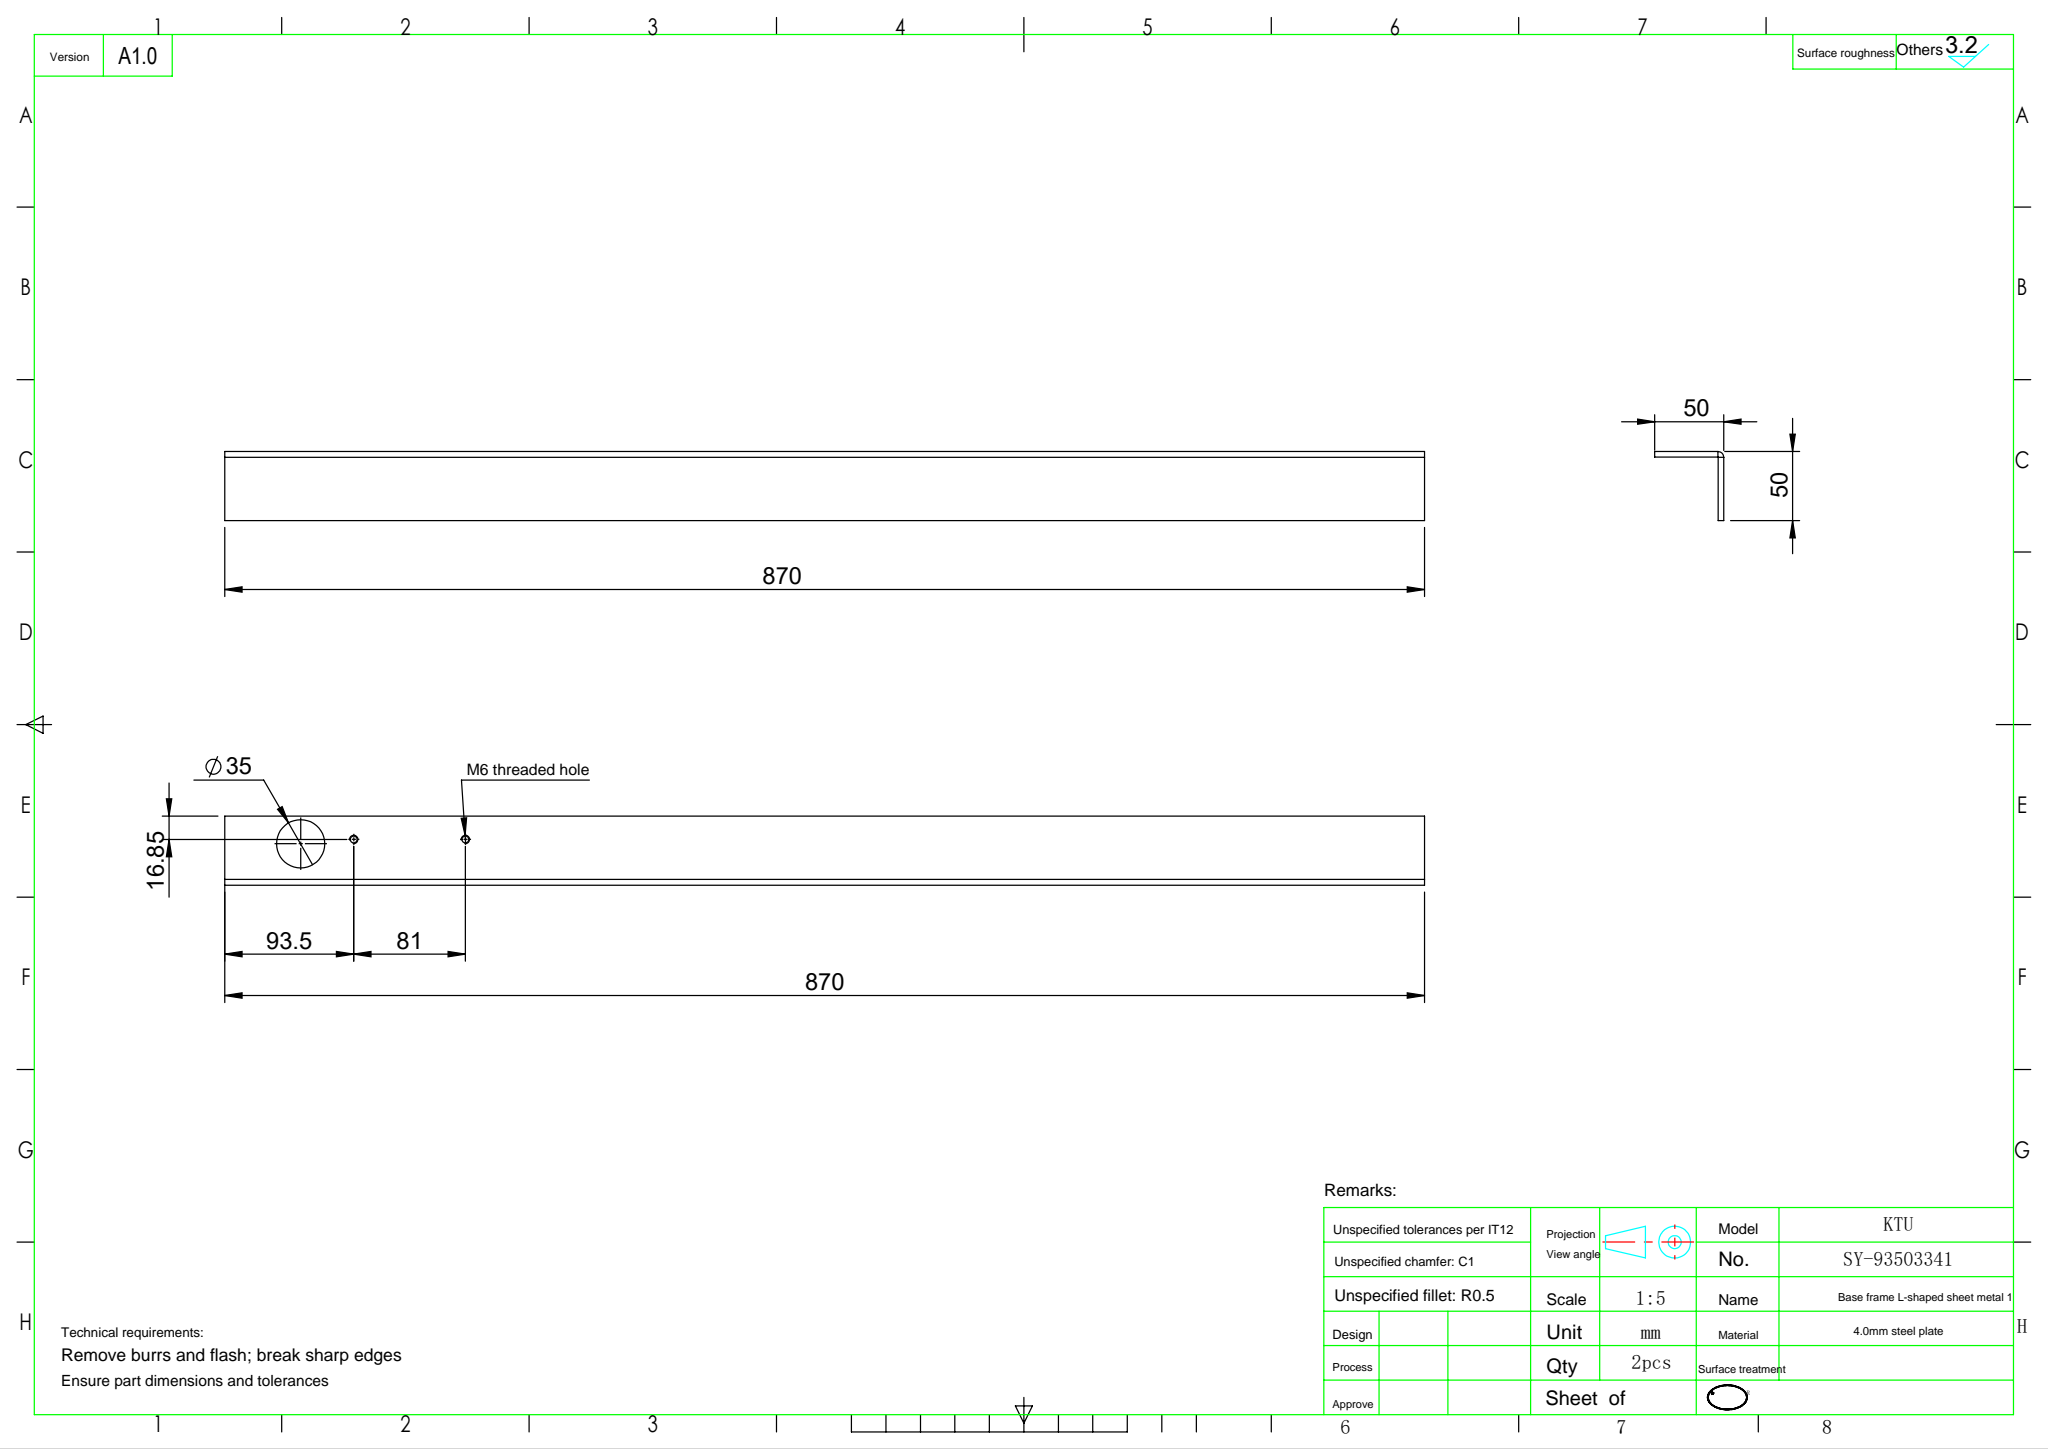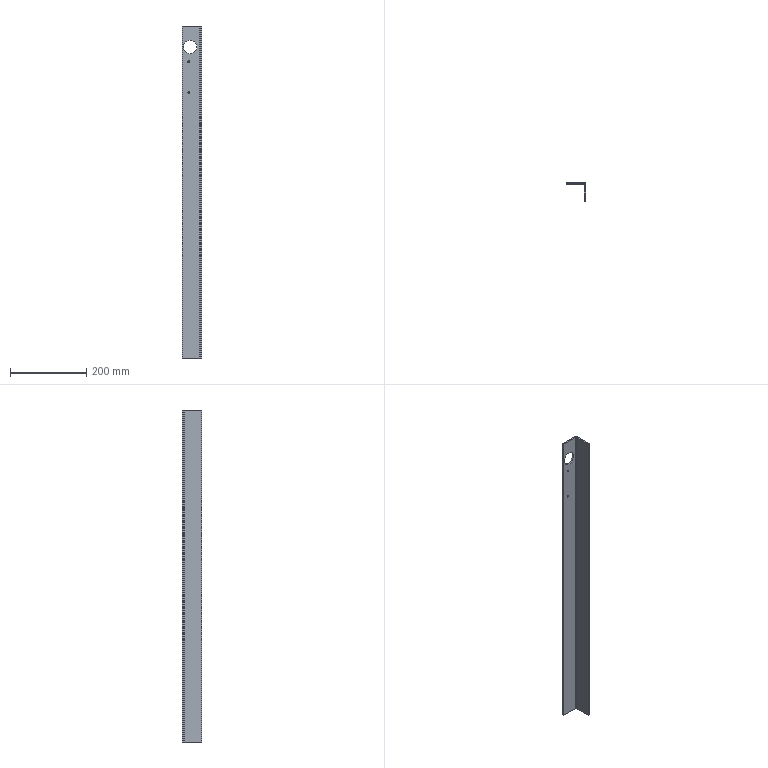Part | SolidWorks | features Cut 1, FlatPattern 1, HoleWzd 1, SMBaseFlange 1, SheetMetal 1 | 1 solid | 20 faces | box 50 x 50 x 870 mm | volume 326788 mm3 | plane 12 | cylinder 8 | commonest cylinder face diameters 5 x4 35 x2 0.4 x1 8.4 x1
STEP:
#1=CARTESIAN_POINT('',(-30.,-4.,797.5));
#2=VERTEX_POINT('',#1);
#3=CARTESIAN_POINT('',(-30.,-4.,832.5));
#4=VERTEX_POINT('',#3);
#5=CARTESIAN_POINT('',(-30.,-4.,815.));
#6=DIRECTION('',(0.,1.,0.));
#7=DIRECTION('',(0.,0.,1.));
#8=AXIS2_PLACEMENT_3D('',#5,#6,#7);
#9=CIRCLE('',#8,17.5);
#10=EDGE_CURVE('',#2,#4,#9,.T.);
#11=ORIENTED_EDGE('',*,*,#10,.F.);
#12=CARTESIAN_POINT('',(-30.,0.,797.5));
#13=VERTEX_POINT('',#12);
#14=CARTESIAN_POINT('',(-30.,-10.,797.5));
#15=DIRECTION('',(0.,1.,0.));
#16=VECTOR('',#15,1000.);
#17=LINE('',#14,#16);
#18=EDGE_CURVE('',#2,#13,#17,.T.);
#19=ORIENTED_EDGE('',*,*,#18,.T.);
#20=CARTESIAN_POINT('',(-30.,0.,832.5));
#21=VERTEX_POINT('',#20);
#22=CARTESIAN_POINT('',(-30.,0.,815.));
#23=DIRECTION('',(0.,1.,0.));
#24=DIRECTION('',(0.,0.,1.));
#25=AXIS2_PLACEMENT_3D('',#22,#23,#24);
#26=CIRCLE('',#25,17.5);
#27=EDGE_CURVE('',#13,#21,#26,.T.);
#28=ORIENTED_EDGE('',*,*,#27,.T.);
#29=CARTESIAN_POINT('',(-30.,-10.,832.5));
#30=DIRECTION('',(0.,1.,0.));
#31=VECTOR('',#30,1000.);
#32=LINE('',#29,#31);
#33=EDGE_CURVE('',#4,#21,#32,.T.);
#34=ORIENTED_EDGE('',*,*,#33,.F.);
#35=EDGE_LOOP('',(#11,#19,#28,#34));
#36=FACE_OUTER_BOUND('',#35,.T.);
#37=CARTESIAN_POINT('',(-30.,-10.,815.));
#38=DIRECTION('',(0.,1.,0.));
#39=DIRECTION('',(0.,0.,1.));
#40=AXIS2_PLACEMENT_3D('',#37,#38,#39);
#41=CYLINDRICAL_SURFACE('',#40,17.5);
#42=ADVANCED_FACE('',(#36),#41,.F.);
#43=CARTESIAN_POINT('',(-33.15,-4.,774.));
#44=VERTEX_POINT('',#43);
#45=CARTESIAN_POINT('',(-33.15,-4.,779.));
#46=VERTEX_POINT('',#45);
#47=CARTESIAN_POINT('',(-33.15,-4.,776.5));
#48=DIRECTION('',(0.,1.,0.));
#49=DIRECTION('',(0.,0.,1.));
#50=AXIS2_PLACEMENT_3D('',#47,#48,#49);
#51=CIRCLE('',#50,2.5);
#52=EDGE_CURVE('',#44,#46,#51,.T.);
#53=ORIENTED_EDGE('',*,*,#52,.F.);
#54=CARTESIAN_POINT('',(-33.15,0.,774.));
#55=VERTEX_POINT('',#54);
#56=CARTESIAN_POINT('',(-33.15,0.,774.));
#57=DIRECTION('',(0.,1.,0.));
#58=VECTOR('',#57,1000.);
#59=LINE('',#56,#58);
#60=EDGE_CURVE('',#44,#55,#59,.T.);
#61=ORIENTED_EDGE('',*,*,#60,.T.);
#62=CARTESIAN_POINT('',(-33.15,0.,779.));
#63=VERTEX_POINT('',#62);
#64=CARTESIAN_POINT('',(-33.15,0.,776.5));
#65=DIRECTION('',(0.,1.,0.));
#66=DIRECTION('',(0.,0.,1.));
#67=AXIS2_PLACEMENT_3D('',#64,#65,#66);
#68=CIRCLE('',#67,2.5);
#69=EDGE_CURVE('',#55,#63,#68,.T.);
#70=ORIENTED_EDGE('',*,*,#69,.T.);
#71=CARTESIAN_POINT('',(-33.15,0.,779.));
#72=DIRECTION('',(0.,1.,0.));
#73=VECTOR('',#72,1000.);
#74=LINE('',#71,#73);
#75=EDGE_CURVE('',#46,#63,#74,.T.);
#76=ORIENTED_EDGE('',*,*,#75,.F.);
#77=EDGE_LOOP('',(#53,#61,#70,#76));
#78=FACE_OUTER_BOUND('',#77,.T.);
#79=CARTESIAN_POINT('',(-33.15,0.,776.5));
#80=DIRECTION('',(0.,1.,0.));
#81=DIRECTION('',(0.,0.,1.));
#82=AXIS2_PLACEMENT_3D('',#79,#80,#81);
#83=CYLINDRICAL_SURFACE('',#82,2.5);
#84=ADVANCED_FACE('',(#78),#83,.F.);
#85=CARTESIAN_POINT('',(-33.15,-4.,693.));
#86=VERTEX_POINT('',#85);
#87=CARTESIAN_POINT('',(-33.15,-4.,698.));
#88=VERTEX_POINT('',#87);
#89=CARTESIAN_POINT('',(-33.15,-4.,695.5));
#90=DIRECTION('',(0.,1.,0.));
#91=DIRECTION('',(0.,0.,1.));
#92=AXIS2_PLACEMENT_3D('',#89,#90,#91);
#93=CIRCLE('',#92,2.5);
#94=EDGE_CURVE('',#86,#88,#93,.T.);
#95=ORIENTED_EDGE('',*,*,#94,.F.);
#96=CARTESIAN_POINT('',(-33.15,0.,693.));
#97=VERTEX_POINT('',#96);
#98=CARTESIAN_POINT('',(-33.15,0.,693.));
#99=DIRECTION('',(0.,1.,0.));
#100=VECTOR('',#99,1000.);
#101=LINE('',#98,#100);
#102=EDGE_CURVE('',#86,#97,#101,.T.);
#103=ORIENTED_EDGE('',*,*,#102,.T.);
#104=CARTESIAN_POINT('',(-33.15,0.,698.));
#105=VERTEX_POINT('',#104);
#106=CARTESIAN_POINT('',(-33.15,0.,695.5));
#107=DIRECTION('',(0.,1.,0.));
#108=DIRECTION('',(0.,0.,1.));
#109=AXIS2_PLACEMENT_3D('',#106,#107,#108);
#110=CIRCLE('',#109,2.5);
#111=EDGE_CURVE('',#97,#105,#110,.T.);
#112=ORIENTED_EDGE('',*,*,#111,.T.);
#113=CARTESIAN_POINT('',(-33.15,0.,698.));
#114=DIRECTION('',(0.,1.,0.));
#115=VECTOR('',#114,1000.);
#116=LINE('',#113,#115);
#117=EDGE_CURVE('',#88,#105,#116,.T.);
#118=ORIENTED_EDGE('',*,*,#117,.F.);
#119=EDGE_LOOP('',(#95,#103,#112,#118));
#120=FACE_OUTER_BOUND('',#119,.T.);
#121=CARTESIAN_POINT('',(-33.15,0.,695.5));
#122=DIRECTION('',(0.,1.,0.));
#123=DIRECTION('',(0.,0.,1.));
#124=AXIS2_PLACEMENT_3D('',#121,#122,#123);
#125=CYLINDRICAL_SURFACE('',#124,2.5);
#126=ADVANCED_FACE('',(#120),#125,.F.);
#127=CARTESIAN_POINT('',(0.,-4.2,870.));
#128=VERTEX_POINT('',#127);
#129=CARTESIAN_POINT('',(-4.,-4.2,870.));
#130=VERTEX_POINT('',#129);
#131=CARTESIAN_POINT('',(0.,-4.2,870.));
#132=DIRECTION('',(-1.,0.,0.));
#133=VECTOR('',#132,1000.);
#134=LINE('',#131,#133);
#135=EDGE_CURVE('',#128,#130,#134,.T.);
#136=ORIENTED_EDGE('',*,*,#135,.F.);
#137=CARTESIAN_POINT('',(-4.2,0.,870.));
#138=VERTEX_POINT('',#137);
#139=CARTESIAN_POINT('',(-4.2,-4.2,870.));
#140=DIRECTION('',(0.,0.,-1.));
#141=DIRECTION('',(1.,0.,0.));
#142=AXIS2_PLACEMENT_3D('',#139,#140,#141);
#143=CIRCLE('',#142,4.2);
#144=EDGE_CURVE('',#138,#128,#143,.T.);
#145=ORIENTED_EDGE('',*,*,#144,.F.);
#146=CARTESIAN_POINT('',(-4.2,-4.,870.));
#147=VERTEX_POINT('',#146);
#148=CARTESIAN_POINT('',(-4.2,-4.,870.));
#149=DIRECTION('',(0.,1.,0.));
#150=VECTOR('',#149,1000.);
#151=LINE('',#148,#150);
#152=EDGE_CURVE('',#147,#138,#151,.T.);
#153=ORIENTED_EDGE('',*,*,#152,.F.);
#154=CARTESIAN_POINT('',(-4.2,-4.2,870.));
#155=DIRECTION('',(0.,0.,-1.));
#156=DIRECTION('',(1.,0.,0.));
#157=AXIS2_PLACEMENT_3D('',#154,#155,#156);
#158=CIRCLE('',#157,0.2);
#159=EDGE_CURVE('',#147,#130,#158,.T.);
#160=ORIENTED_EDGE('',*,*,#159,.T.);
#161=EDGE_LOOP('',(#136,#145,#153,#160));
#162=FACE_OUTER_BOUND('',#161,.T.);
#163=CARTESIAN_POINT('',(0.,-4.2,870.));
#164=DIRECTION('',(0.,0.,1.));
#165=DIRECTION('',(1.,0.,0.));
#166=AXIS2_PLACEMENT_3D('',#163,#164,#165);
#167=PLANE('',#166);
#168=ADVANCED_FACE('',(#162),#167,.T.);
#169=CARTESIAN_POINT('',(0.,-50.,870.));
#170=VERTEX_POINT('',#169);
#171=CARTESIAN_POINT('',(0.,0.,870.));
#172=DIRECTION('',(0.,-1.,0.));
#173=VECTOR('',#172,1000.);
#174=LINE('',#171,#173);
#175=EDGE_CURVE('',#128,#170,#174,.T.);
#176=ORIENTED_EDGE('',*,*,#175,.F.);
#177=ORIENTED_EDGE('',*,*,#135,.T.);
#178=CARTESIAN_POINT('',(-4.,-50.,870.));
#179=VERTEX_POINT('',#178);
#180=CARTESIAN_POINT('',(-4.,0.,870.));
#181=DIRECTION('',(0.,-1.,0.));
#182=VECTOR('',#181,1000.);
#183=LINE('',#180,#182);
#184=EDGE_CURVE('',#130,#179,#183,.T.);
#185=ORIENTED_EDGE('',*,*,#184,.T.);
#186=CARTESIAN_POINT('',(0.,-50.,870.));
#187=DIRECTION('',(-1.,0.,0.));
#188=VECTOR('',#187,1000.);
#189=LINE('',#186,#188);
#190=EDGE_CURVE('',#170,#179,#189,.T.);
#191=ORIENTED_EDGE('',*,*,#190,.F.);
#192=EDGE_LOOP('',(#176,#177,#185,#191));
#193=FACE_OUTER_BOUND('',#192,.T.);
#194=CARTESIAN_POINT('',(-4.2,-4.,870.));
#195=DIRECTION('',(0.,0.,1.));
#196=DIRECTION('',(1.,0.,0.));
#197=AXIS2_PLACEMENT_3D('',#194,#195,#196);
#198=PLANE('',#197);
#199=ADVANCED_FACE('',(#193),#198,.T.);
#200=CARTESIAN_POINT('',(-4.2,0.,0.));
#201=VERTEX_POINT('',#200);
#202=CARTESIAN_POINT('',(-4.2,-4.,0.));
#203=VERTEX_POINT('',#202);
#204=CARTESIAN_POINT('',(-4.2,0.,0.));
#205=DIRECTION('',(0.,-1.,0.));
#206=VECTOR('',#205,1000.);
#207=LINE('',#204,#206);
#208=EDGE_CURVE('',#201,#203,#207,.T.);
#209=ORIENTED_EDGE('',*,*,#208,.F.);
#210=CARTESIAN_POINT('',(0.,-4.2,0.));
#211=VERTEX_POINT('',#210);
#212=CARTESIAN_POINT('',(-4.2,-4.2,0.));
#213=DIRECTION('',(0.,0.,-1.));
#214=DIRECTION('',(1.,0.,0.));
#215=AXIS2_PLACEMENT_3D('',#212,#213,#214);
#216=CIRCLE('',#215,4.2);
#217=EDGE_CURVE('',#201,#211,#216,.T.);
#218=ORIENTED_EDGE('',*,*,#217,.T.);
#219=CARTESIAN_POINT('',(-4.,-4.2,0.));
#220=VERTEX_POINT('',#219);
#221=CARTESIAN_POINT('',(-4.,-4.2,0.));
#222=DIRECTION('',(1.,0.,0.));
#223=VECTOR('',#222,1000.);
#224=LINE('',#221,#223);
#225=EDGE_CURVE('',#220,#211,#224,.T.);
#226=ORIENTED_EDGE('',*,*,#225,.F.);
#227=CARTESIAN_POINT('',(-4.2,-4.2,0.));
#228=DIRECTION('',(0.,0.,-1.));
#229=DIRECTION('',(1.,0.,0.));
#230=AXIS2_PLACEMENT_3D('',#227,#228,#229);
#231=CIRCLE('',#230,0.2);
#232=EDGE_CURVE('',#203,#220,#231,.T.);
#233=ORIENTED_EDGE('',*,*,#232,.F.);
#234=EDGE_LOOP('',(#209,#218,#226,#233));
#235=FACE_OUTER_BOUND('',#234,.T.);
#236=CARTESIAN_POINT('',(-4.2,0.,0.));
#237=DIRECTION('',(0.,0.,-1.));
#238=DIRECTION('',(-1.,0.,0.));
#239=AXIS2_PLACEMENT_3D('',#236,#237,#238);
#240=PLANE('',#239);
#241=ADVANCED_FACE('',(#235),#240,.T.);
#242=CARTESIAN_POINT('',(-50.,0.,0.));
#243=VERTEX_POINT('',#242);
#244=CARTESIAN_POINT('',(-50.,0.,0.));
#245=DIRECTION('',(1.,0.,0.));
#246=VECTOR('',#245,1000.);
#247=LINE('',#244,#246);
#248=EDGE_CURVE('',#243,#201,#247,.T.);
#249=ORIENTED_EDGE('',*,*,#248,.T.);
#250=ORIENTED_EDGE('',*,*,#208,.T.);
#251=CARTESIAN_POINT('',(-50.,-4.,0.));
#252=VERTEX_POINT('',#251);
#253=CARTESIAN_POINT('',(-50.,-4.,0.));
#254=DIRECTION('',(1.,0.,0.));
#255=VECTOR('',#254,1000.);
#256=LINE('',#253,#255);
#257=EDGE_CURVE('',#252,#203,#256,.T.);
#258=ORIENTED_EDGE('',*,*,#257,.F.);
#259=CARTESIAN_POINT('',(-50.,-4.,0.));
#260=DIRECTION('',(0.,1.,0.));
#261=VECTOR('',#260,1000.);
#262=LINE('',#259,#261);
#263=EDGE_CURVE('',#252,#243,#262,.T.);
#264=ORIENTED_EDGE('',*,*,#263,.T.);
#265=EDGE_LOOP('',(#249,#250,#258,#264));
#266=FACE_OUTER_BOUND('',#265,.T.);
#267=CARTESIAN_POINT('',(-4.,-4.2,0.));
#268=DIRECTION('',(0.,0.,-1.));
#269=DIRECTION('',(-1.,0.,0.));
#270=AXIS2_PLACEMENT_3D('',#267,#268,#269);
#271=PLANE('',#270);
#272=ADVANCED_FACE('',(#266),#271,.T.);
#273=CARTESIAN_POINT('',(-4.,-50.,0.));
#274=VERTEX_POINT('',#273);
#275=CARTESIAN_POINT('',(-4.,0.,0.));
#276=DIRECTION('',(0.,-1.,0.));
#277=VECTOR('',#276,1000.);
#278=LINE('',#275,#277);
#279=EDGE_CURVE('',#220,#274,#278,.T.);
#280=ORIENTED_EDGE('',*,*,#279,.T.);
#281=CARTESIAN_POINT('',(-4.,-50.,870.));
#282=DIRECTION('',(0.,0.,-1.));
#283=VECTOR('',#282,1000.);
#284=LINE('',#281,#283);
#285=EDGE_CURVE('',#179,#274,#284,.T.);
#286=ORIENTED_EDGE('',*,*,#285,.F.);
#287=ORIENTED_EDGE('',*,*,#184,.F.);
#288=CARTESIAN_POINT('',(-4.,-4.2,870.));
#289=DIRECTION('',(0.,0.,-1.));
#290=VECTOR('',#289,1000.);
#291=LINE('',#288,#290);
#292=EDGE_CURVE('',#130,#220,#291,.T.);
#293=ORIENTED_EDGE('',*,*,#292,.T.);
#294=EDGE_LOOP('',(#280,#286,#287,#293));
#295=FACE_OUTER_BOUND('',#294,.T.);
#296=CARTESIAN_POINT('',(-4.,0.,870.));
#297=DIRECTION('',(1.,0.,0.));
#298=DIRECTION('',(0.,1.,0.));
#299=AXIS2_PLACEMENT_3D('',#296,#297,#298);
#300=PLANE('',#299);
#301=ADVANCED_FACE('',(#295),#300,.F.);
#302=CARTESIAN_POINT('',(0.,-50.,0.));
#303=VERTEX_POINT('',#302);
#304=CARTESIAN_POINT('',(0.,-50.,0.));
#305=DIRECTION('',(-1.,0.,0.));
#306=VECTOR('',#305,1000.);
#307=LINE('',#304,#306);
#308=EDGE_CURVE('',#303,#274,#307,.T.);
#309=ORIENTED_EDGE('',*,*,#308,.F.);
#310=CARTESIAN_POINT('',(0.,-50.,870.));
#311=DIRECTION('',(0.,0.,-1.));
#312=VECTOR('',#311,1000.);
#313=LINE('',#310,#312);
#314=EDGE_CURVE('',#170,#303,#313,.T.);
#315=ORIENTED_EDGE('',*,*,#314,.F.);
#316=ORIENTED_EDGE('',*,*,#190,.T.);
#317=ORIENTED_EDGE('',*,*,#285,.T.);
#318=EDGE_LOOP('',(#309,#315,#316,#317));
#319=FACE_OUTER_BOUND('',#318,.T.);
#320=CARTESIAN_POINT('',(0.,-50.,870.));
#321=DIRECTION('',(0.,-1.,0.));
#322=DIRECTION('',(0.,0.,-1.));
#323=AXIS2_PLACEMENT_3D('',#320,#321,#322);
#324=PLANE('',#323);
#325=ADVANCED_FACE('',(#319),#324,.T.);
#326=CARTESIAN_POINT('',(0.,0.,0.));
#327=DIRECTION('',(0.,-1.,0.));
#328=VECTOR('',#327,1000.);
#329=LINE('',#326,#328);
#330=EDGE_CURVE('',#211,#303,#329,.T.);
#331=ORIENTED_EDGE('',*,*,#330,.F.);
#332=CARTESIAN_POINT('',(0.,-4.2,870.));
#333=DIRECTION('',(0.,0.,-1.));
#334=VECTOR('',#333,1000.);
#335=LINE('',#332,#334);
#336=EDGE_CURVE('',#128,#211,#335,.T.);
#337=ORIENTED_EDGE('',*,*,#336,.F.);
#338=ORIENTED_EDGE('',*,*,#175,.T.);
#339=ORIENTED_EDGE('',*,*,#314,.T.);
#340=EDGE_LOOP('',(#331,#337,#338,#339));
#341=FACE_OUTER_BOUND('',#340,.T.);
#342=CARTESIAN_POINT('',(0.,0.,870.));
#343=DIRECTION('',(1.,0.,0.));
#344=DIRECTION('',(0.,1.,0.));
#345=AXIS2_PLACEMENT_3D('',#342,#343,#344);
#346=PLANE('',#345);
#347=ADVANCED_FACE('',(#341),#346,.T.);
#348=ORIENTED_EDGE('',*,*,#217,.F.);
#349=CARTESIAN_POINT('',(-4.2,0.,870.));
#350=DIRECTION('',(0.,0.,-1.));
#351=VECTOR('',#350,1000.);
#352=LINE('',#349,#351);
#353=EDGE_CURVE('',#138,#201,#352,.T.);
#354=ORIENTED_EDGE('',*,*,#353,.F.);
#355=ORIENTED_EDGE('',*,*,#144,.T.);
#356=ORIENTED_EDGE('',*,*,#336,.T.);
#357=EDGE_LOOP('',(#348,#354,#355,#356));
#358=FACE_OUTER_BOUND('',#357,.T.);
#359=CARTESIAN_POINT('',(-4.2,-4.2,870.));
#360=DIRECTION('',(0.,0.,-1.));
#361=DIRECTION('',(-1.,0.,0.));
#362=AXIS2_PLACEMENT_3D('',#359,#360,#361);
#363=CYLINDRICAL_SURFACE('',#362,4.2);
#364=ADVANCED_FACE('',(#358),#363,.T.);
#365=CARTESIAN_POINT('',(-30.,0.,815.));
#366=DIRECTION('',(0.,1.,0.));
#367=DIRECTION('',(0.,0.,1.));
#368=AXIS2_PLACEMENT_3D('',#365,#366,#367);
#369=CIRCLE('',#368,17.5);
#370=EDGE_CURVE('',#21,#13,#369,.T.);
#371=ORIENTED_EDGE('',*,*,#370,.F.);
#372=ORIENTED_EDGE('',*,*,#27,.F.);
#373=EDGE_LOOP('',(#371,#372));
#374=FACE_BOUND('',#373,.T.);
#375=CARTESIAN_POINT('',(-33.15,0.,776.5));
#376=DIRECTION('',(0.,1.,0.));
#377=DIRECTION('',(0.,0.,1.));
#378=AXIS2_PLACEMENT_3D('',#375,#376,#377);
#379=CIRCLE('',#378,2.5);
#380=EDGE_CURVE('',#63,#55,#379,.T.);
#381=ORIENTED_EDGE('',*,*,#380,.F.);
#382=ORIENTED_EDGE('',*,*,#69,.F.);
#383=EDGE_LOOP('',(#381,#382));
#384=FACE_BOUND('',#383,.T.);
#385=CARTESIAN_POINT('',(-33.15,0.,695.5));
#386=DIRECTION('',(0.,1.,0.));
#387=DIRECTION('',(0.,0.,1.));
#388=AXIS2_PLACEMENT_3D('',#385,#386,#387);
#389=CIRCLE('',#388,2.5);
#390=EDGE_CURVE('',#105,#97,#389,.T.);
#391=ORIENTED_EDGE('',*,*,#390,.F.);
#392=ORIENTED_EDGE('',*,*,#111,.F.);
#393=EDGE_LOOP('',(#391,#392));
#394=FACE_BOUND('',#393,.T.);
#395=ORIENTED_EDGE('',*,*,#248,.F.);
#396=CARTESIAN_POINT('',(-50.,0.,870.));
#397=VERTEX_POINT('',#396);
#398=CARTESIAN_POINT('',(-50.,0.,870.));
#399=DIRECTION('',(0.,0.,-1.));
#400=VECTOR('',#399,1000.);
#401=LINE('',#398,#400);
#402=EDGE_CURVE('',#397,#243,#401,.T.);
#403=ORIENTED_EDGE('',*,*,#402,.F.);
#404=CARTESIAN_POINT('',(-50.,0.,870.));
#405=DIRECTION('',(1.,0.,0.));
#406=VECTOR('',#405,1000.);
#407=LINE('',#404,#406);
#408=EDGE_CURVE('',#397,#138,#407,.T.);
#409=ORIENTED_EDGE('',*,*,#408,.T.);
#410=ORIENTED_EDGE('',*,*,#353,.T.);
#411=EDGE_LOOP('',(#395,#403,#409,#410));
#412=FACE_OUTER_BOUND('',#411,.T.);
#413=CARTESIAN_POINT('',(-50.,0.,870.));
#414=DIRECTION('',(0.,1.,0.));
#415=DIRECTION('',(0.,0.,1.));
#416=AXIS2_PLACEMENT_3D('',#413,#414,#415);
#417=PLANE('',#416);
#418=ADVANCED_FACE('',(#374,#384,#394,#412),#417,.T.);
#419=ORIENTED_EDGE('',*,*,#263,.F.);
#420=CARTESIAN_POINT('',(-50.,-4.,870.));
#421=VERTEX_POINT('',#420);
#422=CARTESIAN_POINT('',(-50.,-4.,870.));
#423=DIRECTION('',(0.,0.,-1.));
#424=VECTOR('',#423,1000.);
#425=LINE('',#422,#424);
#426=EDGE_CURVE('',#421,#252,#425,.T.);
#427=ORIENTED_EDGE('',*,*,#426,.F.);
#428=CARTESIAN_POINT('',(-50.,-4.,870.));
#429=DIRECTION('',(0.,1.,0.));
#430=VECTOR('',#429,1000.);
#431=LINE('',#428,#430);
#432=EDGE_CURVE('',#421,#397,#431,.T.);
#433=ORIENTED_EDGE('',*,*,#432,.T.);
#434=ORIENTED_EDGE('',*,*,#402,.T.);
#435=EDGE_LOOP('',(#419,#427,#433,#434));
#436=FACE_OUTER_BOUND('',#435,.T.);
#437=CARTESIAN_POINT('',(-50.,-4.,870.));
#438=DIRECTION('',(-1.,0.,0.));
#439=DIRECTION('',(0.,0.,1.));
#440=AXIS2_PLACEMENT_3D('',#437,#438,#439);
#441=PLANE('',#440);
#442=ADVANCED_FACE('',(#436),#441,.T.);
#443=CARTESIAN_POINT('',(-30.,-4.,815.));
#444=DIRECTION('',(0.,1.,0.));
#445=DIRECTION('',(0.,0.,1.));
#446=AXIS2_PLACEMENT_3D('',#443,#444,#445);
#447=CIRCLE('',#446,17.5);
#448=EDGE_CURVE('',#4,#2,#447,.T.);
#449=ORIENTED_EDGE('',*,*,#448,.T.);
#450=ORIENTED_EDGE('',*,*,#10,.T.);
#451=EDGE_LOOP('',(#449,#450));
#452=FACE_BOUND('',#451,.T.);
#453=CARTESIAN_POINT('',(-33.15,-4.,776.5));
#454=DIRECTION('',(0.,1.,0.));
#455=DIRECTION('',(0.,0.,1.));
#456=AXIS2_PLACEMENT_3D('',#453,#454,#455);
#457=CIRCLE('',#456,2.5);
#458=EDGE_CURVE('',#46,#44,#457,.T.);
#459=ORIENTED_EDGE('',*,*,#458,.T.);
#460=ORIENTED_EDGE('',*,*,#52,.T.);
#461=EDGE_LOOP('',(#459,#460));
#462=FACE_BOUND('',#461,.T.);
#463=CARTESIAN_POINT('',(-33.15,-4.,695.5));
#464=DIRECTION('',(0.,1.,0.));
#465=DIRECTION('',(0.,0.,1.));
#466=AXIS2_PLACEMENT_3D('',#463,#464,#465);
#467=CIRCLE('',#466,2.5);
#468=EDGE_CURVE('',#88,#86,#467,.T.);
#469=ORIENTED_EDGE('',*,*,#468,.T.);
#470=ORIENTED_EDGE('',*,*,#94,.T.);
#471=EDGE_LOOP('',(#469,#470));
#472=FACE_BOUND('',#471,.T.);
#473=ORIENTED_EDGE('',*,*,#257,.T.);
#474=CARTESIAN_POINT('',(-4.2,-4.,870.));
#475=DIRECTION('',(0.,0.,-1.));
#476=VECTOR('',#475,1000.);
#477=LINE('',#474,#476);
#478=EDGE_CURVE('',#147,#203,#477,.T.);
#479=ORIENTED_EDGE('',*,*,#478,.F.);
#480=CARTESIAN_POINT('',(-50.,-4.,870.));
#481=DIRECTION('',(1.,0.,0.));
#482=VECTOR('',#481,1000.);
#483=LINE('',#480,#482);
#484=EDGE_CURVE('',#421,#147,#483,.T.);
#485=ORIENTED_EDGE('',*,*,#484,.F.);
#486=ORIENTED_EDGE('',*,*,#426,.T.);
#487=EDGE_LOOP('',(#473,#479,#485,#486));
#488=FACE_OUTER_BOUND('',#487,.T.);
#489=CARTESIAN_POINT('',(-50.,-4.,870.));
#490=DIRECTION('',(0.,1.,0.));
#491=DIRECTION('',(0.,0.,1.));
#492=AXIS2_PLACEMENT_3D('',#489,#490,#491);
#493=PLANE('',#492);
#494=ADVANCED_FACE('',(#452,#462,#472,#488),#493,.F.);
#495=ORIENTED_EDGE('',*,*,#232,.T.);
#496=ORIENTED_EDGE('',*,*,#292,.F.);
#497=ORIENTED_EDGE('',*,*,#159,.F.);
#498=ORIENTED_EDGE('',*,*,#478,.T.);
#499=EDGE_LOOP('',(#495,#496,#497,#498));
#500=FACE_OUTER_BOUND('',#499,.T.);
#501=CARTESIAN_POINT('',(-4.2,-4.2,870.));
#502=DIRECTION('',(0.,0.,-1.));
#503=DIRECTION('',(-1.,0.,0.));
#504=AXIS2_PLACEMENT_3D('',#501,#502,#503);
#505=CYLINDRICAL_SURFACE('',#504,0.2);
#506=ADVANCED_FACE('',(#500),#505,.F.);
#507=ORIENTED_EDGE('',*,*,#484,.T.);
#508=ORIENTED_EDGE('',*,*,#152,.T.);
#509=ORIENTED_EDGE('',*,*,#408,.F.);
#510=ORIENTED_EDGE('',*,*,#432,.F.);
#511=EDGE_LOOP('',(#507,#508,#509,#510));
#512=FACE_OUTER_BOUND('',#511,.T.);
#513=CARTESIAN_POINT('',(-4.2,-4.2,870.));
#514=DIRECTION('',(0.,0.,1.));
#515=DIRECTION('',(1.,0.,0.));
#516=AXIS2_PLACEMENT_3D('',#513,#514,#515);
#517=PLANE('',#516);
#518=ADVANCED_FACE('',(#512),#517,.T.);
#519=ORIENTED_EDGE('',*,*,#279,.F.);
#520=ORIENTED_EDGE('',*,*,#225,.T.);
#521=ORIENTED_EDGE('',*,*,#330,.T.);
#522=ORIENTED_EDGE('',*,*,#308,.T.);
#523=EDGE_LOOP('',(#519,#520,#521,#522));
#524=FACE_OUTER_BOUND('',#523,.T.);
#525=CARTESIAN_POINT('',(-4.2,-4.2,0.));
#526=DIRECTION('',(0.,0.,1.));
#527=DIRECTION('',(1.,0.,0.));
#528=AXIS2_PLACEMENT_3D('',#525,#526,#527);
#529=PLANE('',#528);
#530=ADVANCED_FACE('',(#524),#529,.F.);
#531=ORIENTED_EDGE('',*,*,#102,.F.);
#532=ORIENTED_EDGE('',*,*,#468,.F.);
#533=ORIENTED_EDGE('',*,*,#117,.T.);
#534=ORIENTED_EDGE('',*,*,#390,.T.);
#535=EDGE_LOOP('',(#531,#532,#533,#534));
#536=FACE_OUTER_BOUND('',#535,.T.);
#537=CARTESIAN_POINT('',(-33.15,0.,695.5));
#538=DIRECTION('',(0.,1.,0.));
#539=DIRECTION('',(0.,0.,1.));
#540=AXIS2_PLACEMENT_3D('',#537,#538,#539);
#541=CYLINDRICAL_SURFACE('',#540,2.5);
#542=ADVANCED_FACE('',(#536),#541,.F.);
#543=ORIENTED_EDGE('',*,*,#60,.F.);
#544=ORIENTED_EDGE('',*,*,#458,.F.);
#545=ORIENTED_EDGE('',*,*,#75,.T.);
#546=ORIENTED_EDGE('',*,*,#380,.T.);
#547=EDGE_LOOP('',(#543,#544,#545,#546));
#548=FACE_OUTER_BOUND('',#547,.T.);
#549=CARTESIAN_POINT('',(-33.15,0.,776.5));
#550=DIRECTION('',(0.,1.,0.));
#551=DIRECTION('',(0.,0.,1.));
#552=AXIS2_PLACEMENT_3D('',#549,#550,#551);
#553=CYLINDRICAL_SURFACE('',#552,2.5);
#554=ADVANCED_FACE('',(#548),#553,.F.);
#555=ORIENTED_EDGE('',*,*,#18,.F.);
#556=ORIENTED_EDGE('',*,*,#448,.F.);
#557=ORIENTED_EDGE('',*,*,#33,.T.);
#558=ORIENTED_EDGE('',*,*,#370,.T.);
#559=EDGE_LOOP('',(#555,#556,#557,#558));
#560=FACE_OUTER_BOUND('',#559,.T.);
#561=CARTESIAN_POINT('',(-30.,-10.,815.));
#562=DIRECTION('',(0.,1.,0.));
#563=DIRECTION('',(0.,0.,1.));
#564=AXIS2_PLACEMENT_3D('',#561,#562,#563);
#565=CYLINDRICAL_SURFACE('',#564,17.5);
#566=ADVANCED_FACE('',(#560),#565,.F.);
#567=CLOSED_SHELL('',(#42,#84,#126,#168,#199,#241,#272,#301,#325,#347,#364,#418,#442,#494,#506,#518,#530,#542,#554,#566));
#568=MANIFOLD_SOLID_BREP('',#567);
#569=CARTESIAN_POINT('',(0.,0.,0.));
#570=DIRECTION('',(0.,0.,1.));
#571=DIRECTION('',(1.,0.,0.));
#572=AXIS2_PLACEMENT_3D('',#569,#570,#571);
#573=(LENGTH_UNIT()NAMED_UNIT(*)SI_UNIT(.MILLI.,.METRE.));
#574=UNCERTAINTY_MEASURE_WITH_UNIT(LENGTH_MEASURE(0.00001),#573,'','');
#575=(NAMED_UNIT(*)PLANE_ANGLE_UNIT()SI_UNIT($,.RADIAN.));
#576=(NAMED_UNIT(*)SI_UNIT($,.STERADIAN.)SOLID_ANGLE_UNIT());
#577=(GEOMETRIC_REPRESENTATION_CONTEXT(3)GLOBAL_UNCERTAINTY_ASSIGNED_CONTEXT((#574))GLOBAL_UNIT_ASSIGNED_CONTEXT((#573,#575,#576))REPRESENTATION_CONTEXT('',''));
#578=ADVANCED_BREP_SHAPE_REPRESENTATION('',(#568,#572),#577);